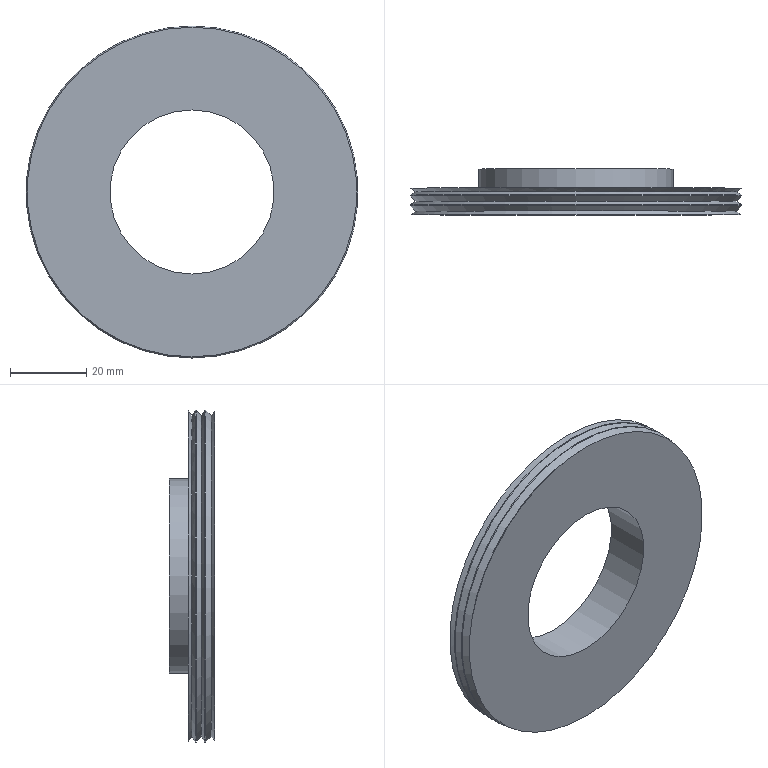Part | NX | features DATUM_CSYS 5, SKETCH 4, EXTRUDE 3, SWP104 1 | 1 solid | 13 faces | box 87 x 12 x 87 mm | volume 33080 mm3 | cone 6 | cylinder 4 | plane 3 | commonest cylinder face diameters 87 x2 43 x1 51 x1
STEP:
#1=CARTESIAN_POINT('',(25.5,-5.,0.));
#2=VERTEX_POINT('',#1);
#3=CARTESIAN_POINT('',(0.,-5.,0.));
#4=DIRECTION('',(0.,-1.,0.));
#5=DIRECTION('',(1.,0.,0.));
#6=AXIS2_PLACEMENT_3D('',#3,#4,#5);
#7=CIRCLE('',#6,25.5);
#8=EDGE_CURVE('',#2,#2,#7,.T.);
#9=ORIENTED_EDGE('',*,*,#8,.T.);
#10=EDGE_LOOP('',(#9));
#11=FACE_BOUND('',#10,.T.);
#12=CARTESIAN_POINT('',(0.,-5.,-43.434));
#13=VERTEX_POINT('',#12);
#14=CARTESIAN_POINT('',(0.,-5.,0.));
#15=DIRECTION('',(0.,-1.,0.));
#16=DIRECTION('',(0.,0.,-1.));
#17=AXIS2_PLACEMENT_3D('',#14,#15,#16);
#18=CIRCLE('',#17,43.434);
#19=EDGE_CURVE('',#13,#13,#18,.T.);
#20=ORIENTED_EDGE('',*,*,#19,.F.);
#21=EDGE_LOOP('',(#20));
#22=FACE_BOUND('',#21,.T.);
#23=CARTESIAN_POINT('',(0.,-5.,0.));
#24=DIRECTION('',(0.,-1.,0.));
#25=DIRECTION('',(0.,0.,-1.));
#26=AXIS2_PLACEMENT_3D('',#23,#24,#25);
#27=PLANE('',#26);
#28=ADVANCED_FACE('',(#11,#22),#27,.F.);
#29=ORIENTED_EDGE('',*,*,#8,.F.);
#30=EDGE_LOOP('',(#29));
#31=FACE_BOUND('',#30,.T.);
#32=CARTESIAN_POINT('',(25.5,0.,0.));
#33=VERTEX_POINT('',#32);
#34=CARTESIAN_POINT('',(0.,0.,0.));
#35=DIRECTION('',(0.,-1.,0.));
#36=DIRECTION('',(1.,0.,0.));
#37=AXIS2_PLACEMENT_3D('',#34,#35,#36);
#38=CIRCLE('',#37,25.5);
#39=EDGE_CURVE('',#33,#33,#38,.T.);
#40=ORIENTED_EDGE('',*,*,#39,.T.);
#41=EDGE_LOOP('',(#40));
#42=FACE_BOUND('',#41,.T.);
#43=CARTESIAN_POINT('',(0.,-5.,0.));
#44=DIRECTION('',(0.,1.,0.));
#45=DIRECTION('',(0.,0.,1.));
#46=AXIS2_PLACEMENT_3D('',#43,#44,#45);
#47=CYLINDRICAL_SURFACE('',#46,25.5);
#48=ADVANCED_FACE('',(#31,#42),#47,.T.);
#49=CARTESIAN_POINT('',(0.,0.,-21.5));
#50=VERTEX_POINT('',#49);
#51=CARTESIAN_POINT('',(0.,0.,0.));
#52=DIRECTION('',(0.,-1.,0.));
#53=DIRECTION('',(0.,0.,-1.));
#54=AXIS2_PLACEMENT_3D('',#51,#52,#53);
#55=CIRCLE('',#54,21.5);
#56=EDGE_CURVE('',#50,#50,#55,.F.);
#57=ORIENTED_EDGE('',*,*,#56,.F.);
#58=EDGE_LOOP('',(#57));
#59=FACE_BOUND('',#58,.T.);
#60=ORIENTED_EDGE('',*,*,#39,.F.);
#61=EDGE_LOOP('',(#60));
#62=FACE_BOUND('',#61,.T.);
#63=CARTESIAN_POINT('',(0.,0.,0.));
#64=DIRECTION('',(0.,-1.,0.));
#65=DIRECTION('',(0.,0.,-1.));
#66=AXIS2_PLACEMENT_3D('',#63,#64,#65);
#67=PLANE('',#66);
#68=ADVANCED_FACE('',(#59,#62),#67,.F.);
#69=CARTESIAN_POINT('',(0.,-5.95,-42.019));
#70=VERTEX_POINT('',#69);
#71=CARTESIAN_POINT('',(0.,-5.95,0.));
#72=DIRECTION('',(0.,-1.,0.));
#73=DIRECTION('',(0.,0.,-1.));
#74=AXIS2_PLACEMENT_3D('',#71,#72,#73);
#75=CIRCLE('',#74,42.019);
#76=EDGE_CURVE('',#70,#70,#75,.F.);
#77=ORIENTED_EDGE('',*,*,#76,.T.);
#78=EDGE_LOOP('',(#77));
#79=FACE_BOUND('',#78,.T.);
#80=ORIENTED_EDGE('',*,*,#19,.T.);
#81=EDGE_LOOP('',(#80));
#82=FACE_BOUND('',#81,.T.);
#83=CARTESIAN_POINT('',(0.,-5.95,0.));
#84=DIRECTION('',(0.,1.,0.));
#85=DIRECTION('',(0.,0.,1.));
#86=AXIS2_PLACEMENT_3D('',#83,#84,#85);
#87=CONICAL_SURFACE('',#86,42.019,0.9795);
#88=ADVANCED_FACE('',(#79,#82),#87,.T.);
#89=ORIENTED_EDGE('',*,*,#76,.F.);
#90=EDGE_LOOP('',(#89));
#91=FACE_BOUND('',#90,.T.);
#92=CARTESIAN_POINT('',(0.,-6.821,-43.5));
#93=VERTEX_POINT('',#92);
#94=CARTESIAN_POINT('',(0.,-6.821,0.));
#95=DIRECTION('',(0.,-1.,0.));
#96=DIRECTION('',(0.,0.,-1.));
#97=AXIS2_PLACEMENT_3D('',#94,#95,#96);
#98=CIRCLE('',#97,43.5);
#99=EDGE_CURVE('',#93,#93,#98,.F.);
#100=ORIENTED_EDGE('',*,*,#99,.T.);
#101=EDGE_LOOP('',(#100));
#102=FACE_BOUND('',#101,.T.);
#103=CARTESIAN_POINT('',(0.,-6.91,0.));
#104=DIRECTION('',(0.,-1.,0.));
#105=DIRECTION('',(0.,0.,-1.));
#106=AXIS2_PLACEMENT_3D('',#103,#104,#105);
#107=CONICAL_SURFACE('',#106,43.651,1.039);
#108=ADVANCED_FACE('',(#91,#102),#107,.T.);
#109=ORIENTED_EDGE('',*,*,#99,.F.);
#110=EDGE_LOOP('',(#109));
#111=FACE_BOUND('',#110,.T.);
#112=CARTESIAN_POINT('',(0.,-7.053,43.5));
#113=VERTEX_POINT('',#112);
#114=CARTESIAN_POINT('',(0.,-7.053,0.));
#115=DIRECTION('',(0.,1.,0.));
#116=DIRECTION('',(0.,0.,1.));
#117=AXIS2_PLACEMENT_3D('',#114,#115,#116);
#118=CIRCLE('',#117,43.5);
#119=EDGE_CURVE('',#113,#113,#118,.F.);
#120=ORIENTED_EDGE('',*,*,#119,.F.);
#121=EDGE_LOOP('',(#120));
#122=FACE_BOUND('',#121,.T.);
#123=CARTESIAN_POINT('',(0.,-12.,0.));
#124=DIRECTION('',(0.,1.,0.));
#125=DIRECTION('',(0.,0.,1.));
#126=AXIS2_PLACEMENT_3D('',#123,#124,#125);
#127=CYLINDRICAL_SURFACE('',#126,43.5);
#128=ADVANCED_FACE('',(#111,#122),#127,.T.);
#129=CARTESIAN_POINT('',(0.,-8.459,-42.017));
#130=VERTEX_POINT('',#129);
#131=CARTESIAN_POINT('',(0.,-8.459,0.));
#132=DIRECTION('',(0.,-1.,0.));
#133=DIRECTION('',(0.,0.,-1.));
#134=AXIS2_PLACEMENT_3D('',#131,#132,#133);
#135=CIRCLE('',#134,42.017);
#136=EDGE_CURVE('',#130,#130,#135,.F.);
#137=ORIENTED_EDGE('',*,*,#136,.F.);
#138=EDGE_LOOP('',(#137));
#139=FACE_BOUND('',#138,.T.);
#140=CARTESIAN_POINT('',(0.,-9.331,-43.5));
#141=VERTEX_POINT('',#140);
#142=CARTESIAN_POINT('',(0.,-9.331,0.));
#143=DIRECTION('',(0.,-1.,0.));
#144=DIRECTION('',(0.,0.,-1.));
#145=AXIS2_PLACEMENT_3D('',#142,#143,#144);
#146=CIRCLE('',#145,43.5);
#147=EDGE_CURVE('',#141,#141,#146,.F.);
#148=ORIENTED_EDGE('',*,*,#147,.T.);
#149=EDGE_LOOP('',(#148));
#150=FACE_BOUND('',#149,.T.);
#151=CARTESIAN_POINT('',(0.,-9.419,0.));
#152=DIRECTION('',(0.,-1.,0.));
#153=DIRECTION('',(0.,0.,-1.));
#154=AXIS2_PLACEMENT_3D('',#151,#152,#153);
#155=CONICAL_SURFACE('',#154,43.651,1.039);
#156=ADVANCED_FACE('',(#139,#150),#155,.T.);
#157=ORIENTED_EDGE('',*,*,#136,.T.);
#158=EDGE_LOOP('',(#157));
#159=FACE_BOUND('',#158,.T.);
#160=ORIENTED_EDGE('',*,*,#119,.T.);
#161=EDGE_LOOP('',(#160));
#162=FACE_BOUND('',#161,.T.);
#163=CARTESIAN_POINT('',(0.,-8.459,0.));
#164=DIRECTION('',(0.,1.,0.));
#165=DIRECTION('',(0.,0.,1.));
#166=AXIS2_PLACEMENT_3D('',#163,#164,#165);
#167=CONICAL_SURFACE('',#166,42.017,0.8121);
#168=ADVANCED_FACE('',(#159,#162),#167,.T.);
#169=ORIENTED_EDGE('',*,*,#147,.F.);
#170=EDGE_LOOP('',(#169));
#171=FACE_BOUND('',#170,.T.);
#172=CARTESIAN_POINT('',(0.,-9.581,43.5));
#173=VERTEX_POINT('',#172);
#174=CARTESIAN_POINT('',(0.,-9.581,0.));
#175=DIRECTION('',(0.,1.,0.));
#176=DIRECTION('',(0.,0.,1.));
#177=AXIS2_PLACEMENT_3D('',#174,#175,#176);
#178=CIRCLE('',#177,43.5);
#179=EDGE_CURVE('',#173,#173,#178,.F.);
#180=ORIENTED_EDGE('',*,*,#179,.F.);
#181=EDGE_LOOP('',(#180));
#182=FACE_BOUND('',#181,.T.);
#183=CARTESIAN_POINT('',(0.,-12.,0.));
#184=DIRECTION('',(0.,1.,0.));
#185=DIRECTION('',(0.,0.,1.));
#186=AXIS2_PLACEMENT_3D('',#183,#184,#185);
#187=CYLINDRICAL_SURFACE('',#186,43.5);
#188=ADVANCED_FACE('',(#171,#182),#187,.T.);
#189=CARTESIAN_POINT('',(0.,-12.,-43.186));
#190=VERTEX_POINT('',#189);
#191=CARTESIAN_POINT('',(0.,-12.,0.));
#192=DIRECTION('',(0.,-1.,0.));
#193=DIRECTION('',(0.,0.,-1.));
#194=AXIS2_PLACEMENT_3D('',#191,#192,#193);
#195=CIRCLE('',#194,43.186);
#196=EDGE_CURVE('',#190,#190,#195,.T.);
#197=ORIENTED_EDGE('',*,*,#196,.F.);
#198=EDGE_LOOP('',(#197));
#199=FACE_BOUND('',#198,.T.);
#200=CARTESIAN_POINT('',(0.,-11.055,-42.121));
#201=VERTEX_POINT('',#200);
#202=CARTESIAN_POINT('',(0.,-11.055,0.));
#203=DIRECTION('',(0.,-1.,0.));
#204=DIRECTION('',(0.,0.,-1.));
#205=AXIS2_PLACEMENT_3D('',#202,#203,#204);
#206=CIRCLE('',#205,42.121);
#207=EDGE_CURVE('',#201,#201,#206,.F.);
#208=ORIENTED_EDGE('',*,*,#207,.F.);
#209=EDGE_LOOP('',(#208));
#210=FACE_BOUND('',#209,.T.);
#211=CARTESIAN_POINT('',(0.,-12.412,0.));
#212=DIRECTION('',(0.,-1.,0.));
#213=DIRECTION('',(0.,0.,-1.));
#214=AXIS2_PLACEMENT_3D('',#211,#212,#213);
#215=CONICAL_SURFACE('',#214,43.651,0.8452);
#216=ADVANCED_FACE('',(#199,#210),#215,.T.);
#217=ORIENTED_EDGE('',*,*,#207,.T.);
#218=EDGE_LOOP('',(#217));
#219=FACE_BOUND('',#218,.T.);
#220=ORIENTED_EDGE('',*,*,#179,.T.);
#221=EDGE_LOOP('',(#220));
#222=FACE_BOUND('',#221,.T.);
#223=CARTESIAN_POINT('',(0.,-11.055,0.));
#224=DIRECTION('',(0.,1.,0.));
#225=DIRECTION('',(0.,0.,1.));
#226=AXIS2_PLACEMENT_3D('',#223,#224,#225);
#227=CONICAL_SURFACE('',#226,42.121,0.7523);
#228=ADVANCED_FACE('',(#219,#222),#227,.T.);
#229=CARTESIAN_POINT('',(0.,-12.,-21.5));
#230=VERTEX_POINT('',#229);
#231=CARTESIAN_POINT('',(0.,-12.,0.));
#232=DIRECTION('',(0.,-1.,0.));
#233=DIRECTION('',(0.,0.,-1.));
#234=AXIS2_PLACEMENT_3D('',#231,#232,#233);
#235=CIRCLE('',#234,21.5);
#236=EDGE_CURVE('',#230,#230,#235,.F.);
#237=ORIENTED_EDGE('',*,*,#236,.T.);
#238=EDGE_LOOP('',(#237));
#239=FACE_BOUND('',#238,.T.);
#240=ORIENTED_EDGE('',*,*,#196,.T.);
#241=EDGE_LOOP('',(#240));
#242=FACE_BOUND('',#241,.T.);
#243=CARTESIAN_POINT('',(0.,-12.,0.));
#244=DIRECTION('',(0.,-1.,0.));
#245=DIRECTION('',(0.,0.,-1.));
#246=AXIS2_PLACEMENT_3D('',#243,#244,#245);
#247=PLANE('',#246);
#248=ADVANCED_FACE('',(#239,#242),#247,.T.);
#249=ORIENTED_EDGE('',*,*,#236,.F.);
#250=EDGE_LOOP('',(#249));
#251=FACE_BOUND('',#250,.T.);
#252=ORIENTED_EDGE('',*,*,#56,.T.);
#253=EDGE_LOOP('',(#252));
#254=FACE_BOUND('',#253,.T.);
#255=CARTESIAN_POINT('',(0.,-22.5,0.));
#256=DIRECTION('',(0.,1.,0.));
#257=DIRECTION('',(0.,0.,1.));
#258=AXIS2_PLACEMENT_3D('',#255,#256,#257);
#259=CYLINDRICAL_SURFACE('',#258,21.5);
#260=ADVANCED_FACE('',(#251,#254),#259,.F.);
#261=CLOSED_SHELL('',(#28,#48,#68,#88,#108,#128,#156,#168,#188,#216,#228,#248,#260));
#262=MANIFOLD_SOLID_BREP('',#261);
#263=(LENGTH_UNIT()NAMED_UNIT(*)SI_UNIT(.MILLI.,.METRE.));
#264=UNCERTAINTY_MEASURE_WITH_UNIT(LENGTH_MEASURE(0.00001),#263,'','');
#265=(NAMED_UNIT(*)PLANE_ANGLE_UNIT()SI_UNIT($,.RADIAN.));
#266=(NAMED_UNIT(*)SI_UNIT($,.STERADIAN.)SOLID_ANGLE_UNIT());
#267=(GEOMETRIC_REPRESENTATION_CONTEXT(3)GLOBAL_UNCERTAINTY_ASSIGNED_CONTEXT((#264))GLOBAL_UNIT_ASSIGNED_CONTEXT((#263,#265,#266))REPRESENTATION_CONTEXT('',''));
#268=ADVANCED_BREP_SHAPE_REPRESENTATION('',(#262),#267);